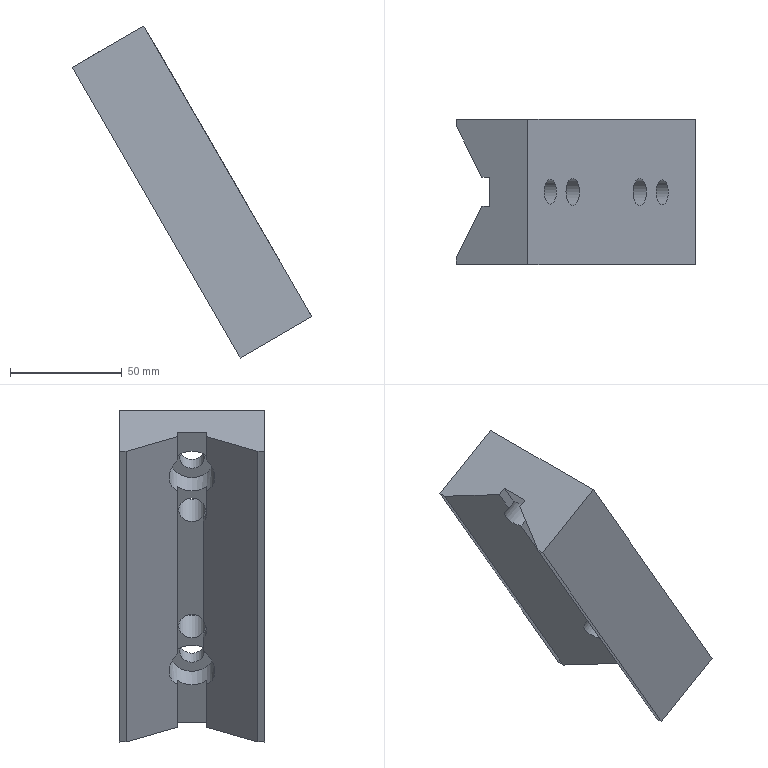Part | NX | features solid 2 | 1 solid | 30 faces | box 107.043 x 65 x 148.404 mm | volume 267589 mm3 | plane 22 | cylinder 8 | commonest cylinder face diameters 11 x2 12 x2 13 x2 20.5 x2
STEP:
#1=CARTESIAN_POINT('',(-1049.455,-56.5,78.567));
#2=VERTEX_POINT('',#1);
#3=CARTESIAN_POINT('',(-1043.418,-56.5,68.11));
#4=VERTEX_POINT('',#3);
#5=CARTESIAN_POINT('',(-1049.455,-56.5,78.567));
#6=DIRECTION('',(0.5,0.,-0.866));
#7=VECTOR('',#6,1000.);
#8=LINE('',#5,#7);
#9=EDGE_CURVE('',#2,#4,#8,.T.);
#10=ORIENTED_EDGE('',*,*,#9,.F.);
#11=CARTESIAN_POINT('',(-1049.455,-43.5,78.567));
#12=VERTEX_POINT('',#11);
#13=CARTESIAN_POINT('',(-1049.455,-82.5,78.567));
#14=DIRECTION('',(0.,-1.,0.));
#15=VECTOR('',#14,1000.);
#16=LINE('',#13,#15);
#17=EDGE_CURVE('',#12,#2,#16,.T.);
#18=ORIENTED_EDGE('',*,*,#17,.F.);
#19=CARTESIAN_POINT('',(-1043.418,-43.5,68.11));
#20=VERTEX_POINT('',#19);
#21=CARTESIAN_POINT('',(-1049.455,-43.5,78.567));
#22=DIRECTION('',(0.5,0.,-0.866));
#23=VECTOR('',#22,1000.);
#24=LINE('',#21,#23);
#25=EDGE_CURVE('',#12,#20,#24,.T.);
#26=ORIENTED_EDGE('',*,*,#25,.T.);
#27=CARTESIAN_POINT('',(-1039.455,-50.,61.247));
#28=DIRECTION('',(-0.866,0.,-0.5));
#29=DIRECTION('',(0.5,0.,-0.866));
#30=AXIS2_PLACEMENT_3D('',#27,#28,#29);
#31=CIRCLE('',#30,10.25);
#32=EDGE_CURVE('',#4,#20,#31,.T.);
#33=ORIENTED_EDGE('',*,*,#32,.F.);
#34=EDGE_LOOP('',(#10,#18,#26,#33));
#35=FACE_BOUND('',#34,.T.);
#36=CARTESIAN_POINT('',(-1049.455,-55.,78.567));
#37=DIRECTION('',(0.866,0.,0.5));
#38=DIRECTION('',(0.,-1.,0.));
#39=AXIS2_PLACEMENT_3D('',#36,#37,#38);
#40=PLANE('',#39);
#41=ADVANCED_FACE('',(#35),#40,.F.);
#42=CARTESIAN_POINT('',(-1046.668,-43.5,66.234));
#43=VERTEX_POINT('',#42);
#44=CARTESIAN_POINT('',(-1052.078,-43.5,63.11));
#45=DIRECTION('',(0.866,0.,0.5));
#46=VECTOR('',#45,1000.);
#47=LINE('',#44,#46);
#48=EDGE_CURVE('',#43,#20,#47,.T.);
#49=ORIENTED_EDGE('',*,*,#48,.T.);
#50=ORIENTED_EDGE('',*,*,#25,.F.);
#51=CARTESIAN_POINT('',(-1052.705,-43.5,76.691));
#52=VERTEX_POINT('',#51);
#53=CARTESIAN_POINT('',(-1050.223,-43.5,78.124));
#54=DIRECTION('',(0.866,0.,0.5));
#55=VECTOR('',#54,1000.);
#56=LINE('',#53,#55);
#57=EDGE_CURVE('',#52,#12,#56,.T.);
#58=ORIENTED_EDGE('',*,*,#57,.F.);
#59=CARTESIAN_POINT('',(-1052.705,-43.5,76.691));
#60=DIRECTION('',(0.5,0.,-0.866));
#61=VECTOR('',#60,1000.);
#62=LINE('',#59,#61);
#63=EDGE_CURVE('',#52,#43,#62,.T.);
#64=ORIENTED_EDGE('',*,*,#63,.T.);
#65=EDGE_LOOP('',(#49,#50,#58,#64));
#66=FACE_BOUND('',#65,.T.);
#67=CARTESIAN_POINT('',(-1050.223,-43.5,78.124));
#68=DIRECTION('',(0.,-1.,0.));
#69=DIRECTION('',(-0.866,0.,-0.5));
#70=AXIS2_PLACEMENT_3D('',#67,#68,#69);
#71=PLANE('',#70);
#72=ADVANCED_FACE('',(#66),#71,.T.);
#73=CARTESIAN_POINT('',(-1052.705,-56.5,76.691));
#74=VERTEX_POINT('',#73);
#75=CARTESIAN_POINT('',(-1046.668,-56.5,66.234));
#76=VERTEX_POINT('',#75);
#77=CARTESIAN_POINT('',(-1052.705,-56.5,76.691));
#78=DIRECTION('',(0.5,0.,-0.866));
#79=VECTOR('',#78,1000.);
#80=LINE('',#77,#79);
#81=EDGE_CURVE('',#74,#76,#80,.T.);
#82=ORIENTED_EDGE('',*,*,#81,.F.);
#83=CARTESIAN_POINT('',(-1050.223,-56.5,78.124));
#84=DIRECTION('',(0.866,0.,0.5));
#85=VECTOR('',#84,1000.);
#86=LINE('',#83,#85);
#87=EDGE_CURVE('',#74,#2,#86,.T.);
#88=ORIENTED_EDGE('',*,*,#87,.T.);
#89=ORIENTED_EDGE('',*,*,#9,.T.);
#90=CARTESIAN_POINT('',(-1052.078,-56.5,63.11));
#91=DIRECTION('',(0.866,0.,0.5));
#92=VECTOR('',#91,1000.);
#93=LINE('',#90,#92);
#94=EDGE_CURVE('',#76,#4,#93,.T.);
#95=ORIENTED_EDGE('',*,*,#94,.F.);
#96=EDGE_LOOP('',(#82,#88,#89,#95));
#97=FACE_BOUND('',#96,.T.);
#98=CARTESIAN_POINT('',(-1050.223,-56.5,78.124));
#99=DIRECTION('',(0.,-1.,0.));
#100=DIRECTION('',(-0.866,0.,-0.5));
#101=AXIS2_PLACEMENT_3D('',#98,#99,#100);
#102=PLANE('',#101);
#103=ADVANCED_FACE('',(#97),#102,.F.);
#104=CARTESIAN_POINT('',(-1038.743,-43.5,52.507));
#105=VERTEX_POINT('',#104);
#106=CARTESIAN_POINT('',(-1039.455,-50.,61.247));
#107=DIRECTION('',(0.75,0.5,0.433));
#108=DIRECTION('',(0.433,-0.866,0.25));
#109=AXIS2_PLACEMENT_3D('',#106,#107,#108);
#110=ELLIPSE('',#109,11.836,10.25);
#111=EDGE_CURVE('',#105,#43,#110,.T.);
#112=ORIENTED_EDGE('',*,*,#111,.T.);
#113=ORIENTED_EDGE('',*,*,#63,.F.);
#114=CARTESIAN_POINT('',(-1064.178,-20.555,70.067));
#115=VERTEX_POINT('',#114);
#116=CARTESIAN_POINT('',(-1064.178,-20.555,70.067));
#117=DIRECTION('',(0.433,-0.866,0.25));
#118=VECTOR('',#117,1000.);
#119=LINE('',#116,#118);
#120=EDGE_CURVE('',#115,#52,#119,.T.);
#121=ORIENTED_EDGE('',*,*,#120,.F.);
#122=CARTESIAN_POINT('',(-989.178,-20.555,-59.836));
#123=VERTEX_POINT('',#122);
#124=CARTESIAN_POINT('',(-1064.178,-20.555,70.067));
#125=DIRECTION('',(0.5,0.,-0.866));
#126=VECTOR('',#125,1000.);
#127=LINE('',#124,#126);
#128=EDGE_CURVE('',#115,#123,#127,.T.);
#129=ORIENTED_EDGE('',*,*,#128,.T.);
#130=CARTESIAN_POINT('',(-977.705,-43.5,-53.213));
#131=VERTEX_POINT('',#130);
#132=CARTESIAN_POINT('',(-987.509,-23.893,-58.873));
#133=DIRECTION('',(-0.433,0.866,-0.25));
#134=VECTOR('',#133,1000.);
#135=LINE('',#132,#134);
#136=EDGE_CURVE('',#123,#131,#135,.F.);
#137=ORIENTED_EDGE('',*,*,#136,.T.);
#138=CARTESIAN_POINT('',(-988.743,-43.5,-34.096));
#139=VERTEX_POINT('',#138);
#140=CARTESIAN_POINT('',(-1052.705,-43.5,76.691));
#141=DIRECTION('',(0.5,0.,-0.866));
#142=VECTOR('',#141,1000.);
#143=LINE('',#140,#142);
#144=EDGE_CURVE('',#139,#131,#143,.T.);
#145=ORIENTED_EDGE('',*,*,#144,.F.);
#146=CARTESIAN_POINT('',(-996.668,-43.5,-20.368));
#147=VERTEX_POINT('',#146);
#148=CARTESIAN_POINT('',(-989.455,-50.,-25.356));
#149=DIRECTION('',(0.75,0.5,0.433));
#150=DIRECTION('',(0.433,-0.866,0.25));
#151=AXIS2_PLACEMENT_3D('',#148,#149,#150);
#152=ELLIPSE('',#151,11.836,10.25);
#153=EDGE_CURVE('',#147,#139,#152,.F.);
#154=ORIENTED_EDGE('',*,*,#153,.F.);
#155=CARTESIAN_POINT('',(-1052.705,-43.5,76.691));
#156=DIRECTION('',(0.5,0.,-0.866));
#157=VECTOR('',#156,1000.);
#158=LINE('',#155,#157);
#159=EDGE_CURVE('',#105,#147,#158,.T.);
#160=ORIENTED_EDGE('',*,*,#159,.F.);
#161=EDGE_LOOP('',(#112,#113,#121,#129,#137,#145,#154,#160));
#162=FACE_BOUND('',#161,.T.);
#163=CARTESIAN_POINT('',(-1064.178,-20.555,70.067));
#164=DIRECTION('',(-0.75,-0.5,-0.433));
#165=DIRECTION('',(-0.433,0.866,-0.25));
#166=AXIS2_PLACEMENT_3D('',#163,#164,#165);
#167=PLANE('',#166);
#168=ADVANCED_FACE('',(#162),#167,.T.);
#169=ORIENTED_EDGE('',*,*,#144,.T.);
#170=CARTESIAN_POINT('',(-974.455,-43.5,-51.336));
#171=VERTEX_POINT('',#170);
#172=CARTESIAN_POINT('',(-976.187,-43.5,-52.336));
#173=DIRECTION('',(-0.866,0.,-0.5));
#174=VECTOR('',#173,1000.);
#175=LINE('',#172,#174);
#176=EDGE_CURVE('',#131,#171,#175,.F.);
#177=ORIENTED_EDGE('',*,*,#176,.T.);
#178=CARTESIAN_POINT('',(-985.493,-43.5,-32.219));
#179=VERTEX_POINT('',#178);
#180=CARTESIAN_POINT('',(-1049.455,-43.5,78.567));
#181=DIRECTION('',(0.5,0.,-0.866));
#182=VECTOR('',#181,1000.);
#183=LINE('',#180,#182);
#184=EDGE_CURVE('',#179,#171,#183,.T.);
#185=ORIENTED_EDGE('',*,*,#184,.F.);
#186=CARTESIAN_POINT('',(-988.743,-43.5,-34.096));
#187=DIRECTION('',(0.866,0.,0.5));
#188=VECTOR('',#187,1000.);
#189=LINE('',#186,#188);
#190=EDGE_CURVE('',#139,#179,#189,.T.);
#191=ORIENTED_EDGE('',*,*,#190,.F.);
#192=EDGE_LOOP('',(#169,#177,#185,#191));
#193=FACE_BOUND('',#192,.T.);
#194=CARTESIAN_POINT('',(-1050.223,-43.5,78.124));
#195=DIRECTION('',(0.,-1.,0.));
#196=DIRECTION('',(-0.866,0.,-0.5));
#197=AXIS2_PLACEMENT_3D('',#194,#195,#196);
#198=PLANE('',#197);
#199=ADVANCED_FACE('',(#193),#198,.T.);
#200=CARTESIAN_POINT('',(-993.929,-55.,-17.607));
#201=VERTEX_POINT('',#200);
#202=CARTESIAN_POINT('',(-996.429,-55.,-19.05));
#203=VERTEX_POINT('',#202);
#204=CARTESIAN_POINT('',(-1002.589,-55.,-22.607));
#205=DIRECTION('',(0.866,0.,0.5));
#206=VECTOR('',#205,1000.);
#207=LINE('',#204,#206);
#208=EDGE_CURVE('',#201,#203,#207,.F.);
#209=ORIENTED_EDGE('',*,*,#208,.T.);
#210=CARTESIAN_POINT('',(-999.879,-55.,-13.075));
#211=VERTEX_POINT('',#210);
#212=CARTESIAN_POINT('',(-1051.955,-55.,77.124));
#213=DIRECTION('',(0.5,0.,-0.866));
#214=VECTOR('',#213,1000.);
#215=LINE('',#212,#214);
#216=EDGE_CURVE('',#211,#203,#215,.T.);
#217=ORIENTED_EDGE('',*,*,#216,.F.);
#218=CARTESIAN_POINT('',(-997.379,-55.,-11.632));
#219=VERTEX_POINT('',#218);
#220=CARTESIAN_POINT('',(-993.049,-55.,-9.132));
#221=DIRECTION('',(-0.866,0.,-0.5));
#222=VECTOR('',#221,1000.);
#223=LINE('',#220,#222);
#224=EDGE_CURVE('',#211,#219,#223,.F.);
#225=ORIENTED_EDGE('',*,*,#224,.T.);
#226=CARTESIAN_POINT('',(-1049.455,-55.,78.567));
#227=DIRECTION('',(0.5,0.,-0.866));
#228=VECTOR('',#227,1000.);
#229=LINE('',#226,#228);
#230=EDGE_CURVE('',#219,#201,#229,.T.);
#231=ORIENTED_EDGE('',*,*,#230,.T.);
#232=EDGE_LOOP('',(#209,#217,#225,#231));
#233=FACE_BOUND('',#232,.T.);
#234=CARTESIAN_POINT('',(-1050.223,-55.,78.124));
#235=DIRECTION('',(0.,-1.,0.));
#236=DIRECTION('',(-0.866,0.,-0.5));
#237=AXIS2_PLACEMENT_3D('',#234,#235,#236);
#238=PLANE('',#237);
#239=ADVANCED_FACE('',(#233),#238,.F.);
#240=CARTESIAN_POINT('',(-988.743,-56.5,-34.096));
#241=VERTEX_POINT('',#240);
#242=CARTESIAN_POINT('',(-985.493,-56.5,-32.219));
#243=VERTEX_POINT('',#242);
#244=CARTESIAN_POINT('',(-994.153,-56.5,-37.219));
#245=DIRECTION('',(0.866,0.,0.5));
#246=VECTOR('',#245,1000.);
#247=LINE('',#244,#246);
#248=EDGE_CURVE('',#241,#243,#247,.T.);
#249=ORIENTED_EDGE('',*,*,#248,.T.);
#250=CARTESIAN_POINT('',(-974.455,-56.5,-51.336));
#251=VERTEX_POINT('',#250);
#252=CARTESIAN_POINT('',(-1049.455,-56.5,78.567));
#253=DIRECTION('',(0.5,0.,-0.866));
#254=VECTOR('',#253,1000.);
#255=LINE('',#252,#254);
#256=EDGE_CURVE('',#243,#251,#255,.T.);
#257=ORIENTED_EDGE('',*,*,#256,.T.);
#258=CARTESIAN_POINT('',(-977.705,-56.5,-53.213));
#259=VERTEX_POINT('',#258);
#260=CARTESIAN_POINT('',(-976.187,-56.5,-52.336));
#261=DIRECTION('',(-0.866,0.,-0.5));
#262=VECTOR('',#261,1000.);
#263=LINE('',#260,#262);
#264=EDGE_CURVE('',#259,#251,#263,.F.);
#265=ORIENTED_EDGE('',*,*,#264,.F.);
#266=CARTESIAN_POINT('',(-1052.705,-56.5,76.691));
#267=DIRECTION('',(0.5,0.,-0.866));
#268=VECTOR('',#267,1000.);
#269=LINE('',#266,#268);
#270=EDGE_CURVE('',#241,#259,#269,.T.);
#271=ORIENTED_EDGE('',*,*,#270,.F.);
#272=EDGE_LOOP('',(#249,#257,#265,#271));
#273=FACE_BOUND('',#272,.T.);
#274=CARTESIAN_POINT('',(-1050.223,-56.5,78.124));
#275=DIRECTION('',(0.,-1.,0.));
#276=DIRECTION('',(-0.866,0.,-0.5));
#277=AXIS2_PLACEMENT_3D('',#274,#275,#276);
#278=PLANE('',#277);
#279=ADVANCED_FACE('',(#273),#278,.F.);
#280=CARTESIAN_POINT('',(-1038.743,-56.5,52.507));
#281=VERTEX_POINT('',#280);
#282=CARTESIAN_POINT('',(-1032.705,-56.5,42.05));
#283=VERTEX_POINT('',#282);
#284=CARTESIAN_POINT('',(-1052.705,-56.5,76.691));
#285=DIRECTION('',(0.5,0.,-0.866));
#286=VECTOR('',#285,1000.);
#287=LINE('',#284,#286);
#288=EDGE_CURVE('',#281,#283,#287,.T.);
#289=ORIENTED_EDGE('',*,*,#288,.T.);
#290=CARTESIAN_POINT('',(-1029.879,-55.,38.886));
#291=VERTEX_POINT('',#290);
#292=CARTESIAN_POINT('',(-1029.455,-50.,43.926));
#293=DIRECTION('',(-0.75,0.5,-0.433));
#294=DIRECTION('',(-0.433,-0.866,-0.25));
#295=AXIS2_PLACEMENT_3D('',#292,#293,#294);
#296=ELLIPSE('',#295,7.506,6.5);
#297=EDGE_CURVE('',#283,#291,#296,.F.);
#298=ORIENTED_EDGE('',*,*,#297,.T.);
#299=CARTESIAN_POINT('',(-1004.032,-55.,-5.882));
#300=VERTEX_POINT('',#299);
#301=CARTESIAN_POINT('',(-1051.955,-55.,77.124));
#302=DIRECTION('',(0.5,0.,-0.866));
#303=VECTOR('',#302,1000.);
#304=LINE('',#301,#303);
#305=EDGE_CURVE('',#291,#300,#304,.T.);
#306=ORIENTED_EDGE('',*,*,#305,.T.);
#307=CARTESIAN_POINT('',(-999.455,-50.,-8.035));
#308=DIRECTION('',(-0.75,0.5,-0.433));
#309=DIRECTION('',(-0.433,-0.866,-0.25));
#310=AXIS2_PLACEMENT_3D('',#307,#308,#309);
#311=ELLIPSE('',#310,7.506,6.5);
#312=EDGE_CURVE('',#300,#211,#311,.F.);
#313=ORIENTED_EDGE('',*,*,#312,.T.);
#314=ORIENTED_EDGE('',*,*,#216,.T.);
#315=CARTESIAN_POINT('',(-989.455,-50.,-25.356));
#316=DIRECTION('',(-0.75,0.5,-0.433));
#317=DIRECTION('',(0.433,0.866,0.25));
#318=AXIS2_PLACEMENT_3D('',#315,#316,#317);
#319=ELLIPSE('',#318,11.836,10.25);
#320=EDGE_CURVE('',#203,#241,#319,.F.);
#321=ORIENTED_EDGE('',*,*,#320,.T.);
#322=ORIENTED_EDGE('',*,*,#270,.T.);
#323=CARTESIAN_POINT('',(-989.178,-79.445,-59.836));
#324=VERTEX_POINT('',#323);
#325=CARTESIAN_POINT('',(-962.701,-26.491,-44.55));
#326=DIRECTION('',(-0.433,-0.866,-0.25));
#327=VECTOR('',#326,1000.);
#328=LINE('',#325,#327);
#329=EDGE_CURVE('',#324,#259,#328,.F.);
#330=ORIENTED_EDGE('',*,*,#329,.F.);
#331=CARTESIAN_POINT('',(-1064.178,-79.445,70.067));
#332=VERTEX_POINT('',#331);
#333=CARTESIAN_POINT('',(-1064.178,-79.445,70.067));
#334=DIRECTION('',(-0.5,0.,0.866));
#335=VECTOR('',#334,1000.);
#336=LINE('',#333,#335);
#337=EDGE_CURVE('',#332,#324,#336,.F.);
#338=ORIENTED_EDGE('',*,*,#337,.F.);
#339=CARTESIAN_POINT('',(-1064.178,-79.445,70.067));
#340=DIRECTION('',(0.433,0.866,0.25));
#341=VECTOR('',#340,1000.);
#342=LINE('',#339,#341);
#343=EDGE_CURVE('',#332,#74,#342,.T.);
#344=ORIENTED_EDGE('',*,*,#343,.T.);
#345=ORIENTED_EDGE('',*,*,#81,.T.);
#346=CARTESIAN_POINT('',(-1039.455,-50.,61.247));
#347=DIRECTION('',(-0.75,0.5,-0.433));
#348=DIRECTION('',(0.433,0.866,0.25));
#349=AXIS2_PLACEMENT_3D('',#346,#347,#348);
#350=ELLIPSE('',#349,11.836,10.25);
#351=EDGE_CURVE('',#281,#76,#350,.T.);
#352=ORIENTED_EDGE('',*,*,#351,.F.);
#353=EDGE_LOOP('',(#289,#298,#306,#313,#314,#321,#322,#330,#338,#344,#345,#352));
#354=FACE_BOUND('',#353,.T.);
#355=CARTESIAN_POINT('',(-1064.178,-79.445,70.067));
#356=DIRECTION('',(0.75,-0.5,0.433));
#357=DIRECTION('',(-0.433,-0.866,-0.25));
#358=AXIS2_PLACEMENT_3D('',#355,#356,#357);
#359=PLANE('',#358);
#360=ADVANCED_FACE('',(#354),#359,.F.);
#361=CARTESIAN_POINT('',(-989.455,-50.,-25.356));
#362=DIRECTION('',(-0.866,0.,-0.5));
#363=DIRECTION('',(0.5,0.,-0.866));
#364=AXIS2_PLACEMENT_3D('',#361,#362,#363);
#365=CIRCLE('',#364,10.25);
#366=EDGE_CURVE('',#243,#179,#365,.F.);
#367=ORIENTED_EDGE('',*,*,#366,.T.);
#368=ORIENTED_EDGE('',*,*,#184,.T.);
#369=CARTESIAN_POINT('',(-974.455,-17.5,-51.336));
#370=DIRECTION('',(0.,-1.,0.));
#371=VECTOR('',#370,1000.);
#372=LINE('',#369,#371);
#373=EDGE_CURVE('',#251,#171,#372,.F.);
#374=ORIENTED_EDGE('',*,*,#373,.F.);
#375=ORIENTED_EDGE('',*,*,#256,.F.);
#376=EDGE_LOOP('',(#367,#368,#374,#375));
#377=FACE_BOUND('',#376,.T.);
#378=CARTESIAN_POINT('',(-1049.455,-55.,78.567));
#379=DIRECTION('',(0.866,0.,0.5));
#380=DIRECTION('',(0.,-1.,0.));
#381=AXIS2_PLACEMENT_3D('',#378,#379,#380);
#382=PLANE('',#381);
#383=ADVANCED_FACE('',(#377),#382,.F.);
#384=CARTESIAN_POINT('',(-1026.455,-50.,38.73));
#385=VERTEX_POINT('',#384);
#386=CARTESIAN_POINT('',(-1029.455,-50.,43.926));
#387=DIRECTION('',(-0.866,0.,-0.5));
#388=DIRECTION('',(0.5,0.,-0.866));
#389=AXIS2_PLACEMENT_3D('',#386,#387,#388);
#390=CIRCLE('',#389,6.);
#391=EDGE_CURVE('',#385,#385,#390,.T.);
#392=ORIENTED_EDGE('',*,*,#391,.F.);
#393=EDGE_LOOP('',(#392));
#394=FACE_BOUND('',#393,.T.);
#395=CARTESIAN_POINT('',(-996.455,-50.,-13.231));
#396=VERTEX_POINT('',#395);
#397=CARTESIAN_POINT('',(-999.455,-50.,-8.035));
#398=DIRECTION('',(-0.866,0.,-0.5));
#399=DIRECTION('',(0.5,0.,-0.866));
#400=AXIS2_PLACEMENT_3D('',#397,#398,#399);
#401=CIRCLE('',#400,6.);
#402=EDGE_CURVE('',#396,#396,#401,.T.);
#403=ORIENTED_EDGE('',*,*,#402,.F.);
#404=EDGE_LOOP('',(#403));
#405=FACE_BOUND('',#404,.T.);
#406=CARTESIAN_POINT('',(-1035.493,-43.5,54.383));
#407=VERTEX_POINT('',#406);
#408=CARTESIAN_POINT('',(-993.418,-43.5,-18.492));
#409=VERTEX_POINT('',#408);
#410=CARTESIAN_POINT('',(-1049.455,-43.5,78.567));
#411=DIRECTION('',(0.5,0.,-0.866));
#412=VECTOR('',#411,1000.);
#413=LINE('',#410,#412);
#414=EDGE_CURVE('',#407,#409,#413,.T.);
#415=ORIENTED_EDGE('',*,*,#414,.T.);
#416=CARTESIAN_POINT('',(-989.455,-50.,-25.356));
#417=DIRECTION('',(-0.866,0.,-0.5));
#418=DIRECTION('',(0.5,0.,-0.866));
#419=AXIS2_PLACEMENT_3D('',#416,#417,#418);
#420=CIRCLE('',#419,10.25);
#421=EDGE_CURVE('',#409,#201,#420,.F.);
#422=ORIENTED_EDGE('',*,*,#421,.T.);
#423=ORIENTED_EDGE('',*,*,#230,.F.);
#424=CARTESIAN_POINT('',(-1001.532,-55.,-4.438));
#425=VERTEX_POINT('',#424);
#426=CARTESIAN_POINT('',(-999.455,-50.,-8.035));
#427=DIRECTION('',(-0.866,0.,-0.5));
#428=DIRECTION('',(0.5,0.,-0.866));
#429=AXIS2_PLACEMENT_3D('',#426,#427,#428);
#430=CIRCLE('',#429,6.5);
#431=EDGE_CURVE('',#219,#425,#430,.T.);
#432=ORIENTED_EDGE('',*,*,#431,.T.);
#433=CARTESIAN_POINT('',(-1027.379,-55.,40.329));
#434=VERTEX_POINT('',#433);
#435=CARTESIAN_POINT('',(-1049.455,-55.,78.567));
#436=DIRECTION('',(0.5,0.,-0.866));
#437=VECTOR('',#436,1000.);
#438=LINE('',#435,#437);
#439=EDGE_CURVE('',#434,#425,#438,.T.);
#440=ORIENTED_EDGE('',*,*,#439,.F.);
#441=CARTESIAN_POINT('',(-1029.455,-56.5,43.926));
#442=VERTEX_POINT('',#441);
#443=CARTESIAN_POINT('',(-1029.455,-50.,43.926));
#444=DIRECTION('',(-0.866,0.,-0.5));
#445=DIRECTION('',(0.5,0.,-0.866));
#446=AXIS2_PLACEMENT_3D('',#443,#444,#445);
#447=CIRCLE('',#446,6.5);
#448=EDGE_CURVE('',#434,#442,#447,.T.);
#449=ORIENTED_EDGE('',*,*,#448,.T.);
#450=CARTESIAN_POINT('',(-1035.493,-56.5,54.383));
#451=VERTEX_POINT('',#450);
#452=CARTESIAN_POINT('',(-1049.455,-56.5,78.567));
#453=DIRECTION('',(0.5,0.,-0.866));
#454=VECTOR('',#453,1000.);
#455=LINE('',#452,#454);
#456=EDGE_CURVE('',#451,#442,#455,.T.);
#457=ORIENTED_EDGE('',*,*,#456,.F.);
#458=CARTESIAN_POINT('',(-1039.455,-50.,61.247));
#459=DIRECTION('',(-0.866,0.,-0.5));
#460=DIRECTION('',(0.5,0.,-0.866));
#461=AXIS2_PLACEMENT_3D('',#458,#459,#460);
#462=CIRCLE('',#461,10.25);
#463=EDGE_CURVE('',#407,#451,#462,.T.);
#464=ORIENTED_EDGE('',*,*,#463,.F.);
#465=EDGE_LOOP('',(#415,#422,#423,#432,#440,#449,#457,#464));
#466=FACE_BOUND('',#465,.T.);
#467=CARTESIAN_POINT('',(-1049.455,-55.,78.567));
#468=DIRECTION('',(0.866,0.,0.5));
#469=DIRECTION('',(0.,-1.,0.));
#470=AXIS2_PLACEMENT_3D('',#467,#468,#469);
#471=PLANE('',#470);
#472=ADVANCED_FACE('',(#394,#405,#466),#471,.F.);
#473=CARTESIAN_POINT('',(-1022.135,-44.5,71.247));
#474=VERTEX_POINT('',#473);
#475=CARTESIAN_POINT('',(-1022.135,-50.,71.247));
#476=DIRECTION('',(-0.866,0.,-0.5));
#477=DIRECTION('',(0.,1.,0.));
#478=AXIS2_PLACEMENT_3D('',#475,#476,#477);
#479=CIRCLE('',#478,5.5);
#480=EDGE_CURVE('',#474,#474,#479,.T.);
#481=ORIENTED_EDGE('',*,*,#480,.T.);
#482=EDGE_LOOP('',(#481));
#483=FACE_BOUND('',#482,.T.);
#484=CARTESIAN_POINT('',(-957.135,-82.5,-41.336));
#485=VERTEX_POINT('',#484);
#486=CARTESIAN_POINT('',(-957.135,-17.5,-41.336));
#487=VERTEX_POINT('',#486);
#488=CARTESIAN_POINT('',(-957.135,-17.5,-41.336));
#489=DIRECTION('',(0.,-1.,0.));
#490=VECTOR('',#489,1000.);
#491=LINE('',#488,#490);
#492=EDGE_CURVE('',#485,#487,#491,.F.);
#493=ORIENTED_EDGE('',*,*,#492,.T.);
#494=CARTESIAN_POINT('',(-1032.135,-17.5,88.567));
#495=VERTEX_POINT('',#494);
#496=CARTESIAN_POINT('',(-1032.135,-17.5,88.567));
#497=DIRECTION('',(0.5,0.,-0.866));
#498=VECTOR('',#497,1000.);
#499=LINE('',#496,#498);
#500=EDGE_CURVE('',#495,#487,#499,.T.);
#501=ORIENTED_EDGE('',*,*,#500,.F.);
#502=CARTESIAN_POINT('',(-1032.135,-82.5,88.567));
#503=VERTEX_POINT('',#502);
#504=CARTESIAN_POINT('',(-1032.135,-50.,88.567));
#505=DIRECTION('',(0.,-1.,0.));
#506=VECTOR('',#505,1000.);
#507=LINE('',#504,#506);
#508=EDGE_CURVE('',#495,#503,#507,.T.);
#509=ORIENTED_EDGE('',*,*,#508,.T.);
#510=CARTESIAN_POINT('',(-1032.135,-82.5,88.567));
#511=DIRECTION('',(0.5,0.,-0.866));
#512=VECTOR('',#511,1000.);
#513=LINE('',#510,#512);
#514=EDGE_CURVE('',#503,#485,#513,.T.);
#515=ORIENTED_EDGE('',*,*,#514,.T.);
#516=EDGE_LOOP('',(#493,#501,#509,#515));
#517=FACE_BOUND('',#516,.T.);
#518=CARTESIAN_POINT('',(-1009.135,-50.,48.73));
#519=VERTEX_POINT('',#518);
#520=CARTESIAN_POINT('',(-1012.135,-50.,53.926));
#521=DIRECTION('',(-0.866,0.,-0.5));
#522=DIRECTION('',(0.5,0.,-0.866));
#523=AXIS2_PLACEMENT_3D('',#520,#521,#522);
#524=CIRCLE('',#523,6.);
#525=EDGE_CURVE('',#519,#519,#524,.F.);
#526=ORIENTED_EDGE('',*,*,#525,.F.);
#527=EDGE_LOOP('',(#526));
#528=FACE_BOUND('',#527,.T.);
#529=CARTESIAN_POINT('',(-979.135,-50.,-3.231));
#530=VERTEX_POINT('',#529);
#531=CARTESIAN_POINT('',(-982.135,-50.,1.965));
#532=DIRECTION('',(-0.866,0.,-0.5));
#533=DIRECTION('',(0.5,0.,-0.866));
#534=AXIS2_PLACEMENT_3D('',#531,#532,#533);
#535=CIRCLE('',#534,6.);
#536=EDGE_CURVE('',#530,#530,#535,.F.);
#537=ORIENTED_EDGE('',*,*,#536,.F.);
#538=EDGE_LOOP('',(#537));
#539=FACE_BOUND('',#538,.T.);
#540=CARTESIAN_POINT('',(-972.135,-44.5,-15.356));
#541=VERTEX_POINT('',#540);
#542=CARTESIAN_POINT('',(-972.135,-50.,-15.356));
#543=DIRECTION('',(0.866,0.,0.5));
#544=DIRECTION('',(0.,1.,0.));
#545=AXIS2_PLACEMENT_3D('',#542,#543,#544);
#546=CIRCLE('',#545,5.5);
#547=EDGE_CURVE('',#541,#541,#546,.T.);
#548=ORIENTED_EDGE('',*,*,#547,.F.);
#549=EDGE_LOOP('',(#548));
#550=FACE_BOUND('',#549,.T.);
#551=CARTESIAN_POINT('',(-1032.135,-50.,88.567));
#552=DIRECTION('',(0.866,0.,0.5));
#553=DIRECTION('',(0.,-1.,0.));
#554=AXIS2_PLACEMENT_3D('',#551,#552,#553);
#555=PLANE('',#554);
#556=ADVANCED_FACE('',(#483,#517,#528,#539,#550),#555,.T.);
#557=CARTESIAN_POINT('',(-997.202,-55.,-1.938));
#558=DIRECTION('',(-0.866,0.,-0.5));
#559=VECTOR('',#558,1000.);
#560=LINE('',#557,#559);
#561=EDGE_CURVE('',#425,#300,#560,.T.);
#562=ORIENTED_EDGE('',*,*,#561,.T.);
#563=ORIENTED_EDGE('',*,*,#305,.F.);
#564=CARTESIAN_POINT('',(-1023.049,-55.,42.829));
#565=DIRECTION('',(-0.866,0.,-0.5));
#566=VECTOR('',#565,1000.);
#567=LINE('',#564,#566);
#568=EDGE_CURVE('',#291,#434,#567,.F.);
#569=ORIENTED_EDGE('',*,*,#568,.T.);
#570=ORIENTED_EDGE('',*,*,#439,.T.);
#571=EDGE_LOOP('',(#562,#563,#569,#570));
#572=FACE_BOUND('',#571,.T.);
#573=CARTESIAN_POINT('',(-1050.223,-55.,78.124));
#574=DIRECTION('',(0.,-1.,0.));
#575=DIRECTION('',(-0.866,0.,-0.5));
#576=AXIS2_PLACEMENT_3D('',#573,#574,#575);
#577=PLANE('',#576);
#578=ADVANCED_FACE('',(#572),#577,.F.);
#579=CARTESIAN_POINT('',(-1044.153,-43.5,49.383));
#580=DIRECTION('',(0.866,0.,0.5));
#581=VECTOR('',#580,1000.);
#582=LINE('',#579,#581);
#583=EDGE_CURVE('',#407,#105,#582,.F.);
#584=ORIENTED_EDGE('',*,*,#583,.T.);
#585=ORIENTED_EDGE('',*,*,#159,.T.);
#586=CARTESIAN_POINT('',(-989.088,-43.5,-15.992));
#587=DIRECTION('',(0.866,0.,0.5));
#588=VECTOR('',#587,1000.);
#589=LINE('',#586,#588);
#590=EDGE_CURVE('',#409,#147,#589,.F.);
#591=ORIENTED_EDGE('',*,*,#590,.F.);
#592=ORIENTED_EDGE('',*,*,#414,.F.);
#593=EDGE_LOOP('',(#584,#585,#591,#592));
#594=FACE_BOUND('',#593,.T.);
#595=CARTESIAN_POINT('',(-1050.223,-43.5,78.124));
#596=DIRECTION('',(0.,-1.,0.));
#597=DIRECTION('',(-0.866,0.,-0.5));
#598=AXIS2_PLACEMENT_3D('',#595,#596,#597);
#599=PLANE('',#598);
#600=ADVANCED_FACE('',(#594),#599,.T.);
#601=ORIENTED_EDGE('',*,*,#456,.T.);
#602=CARTESIAN_POINT('',(-1028.54,-56.5,44.455));
#603=DIRECTION('',(-0.866,0.,-0.5));
#604=VECTOR('',#603,1000.);
#605=LINE('',#602,#604);
#606=EDGE_CURVE('',#442,#283,#605,.T.);
#607=ORIENTED_EDGE('',*,*,#606,.T.);
#608=ORIENTED_EDGE('',*,*,#288,.F.);
#609=CARTESIAN_POINT('',(-1044.153,-56.5,49.383));
#610=DIRECTION('',(0.866,0.,0.5));
#611=VECTOR('',#610,1000.);
#612=LINE('',#609,#611);
#613=EDGE_CURVE('',#451,#281,#612,.F.);
#614=ORIENTED_EDGE('',*,*,#613,.F.);
#615=EDGE_LOOP('',(#601,#607,#608,#614));
#616=FACE_BOUND('',#615,.T.);
#617=CARTESIAN_POINT('',(-1050.223,-56.5,78.124));
#618=DIRECTION('',(0.,-1.,0.));
#619=DIRECTION('',(-0.866,0.,-0.5));
#620=AXIS2_PLACEMENT_3D('',#617,#618,#619);
#621=PLANE('',#620);
#622=ADVANCED_FACE('',(#616),#621,.F.);
#623=CARTESIAN_POINT('',(-989.178,-17.5,-59.836));
#624=VERTEX_POINT('',#623);
#625=CARTESIAN_POINT('',(-989.178,-17.5,-59.836));
#626=DIRECTION('',(0.,1.,0.));
#627=VECTOR('',#626,1000.);
#628=LINE('',#625,#627);
#629=EDGE_CURVE('',#624,#123,#628,.F.);
#630=ORIENTED_EDGE('',*,*,#629,.T.);
#631=ORIENTED_EDGE('',*,*,#128,.F.);
#632=CARTESIAN_POINT('',(-1064.178,-17.5,70.067));
#633=VERTEX_POINT('',#632);
#634=CARTESIAN_POINT('',(-1064.178,-17.5,70.067));
#635=DIRECTION('',(0.,-1.,0.));
#636=VECTOR('',#635,1000.);
#637=LINE('',#634,#636);
#638=EDGE_CURVE('',#633,#115,#637,.T.);
#639=ORIENTED_EDGE('',*,*,#638,.F.);
#640=CARTESIAN_POINT('',(-1064.178,-17.5,70.067));
#641=DIRECTION('',(0.5,0.,-0.866));
#642=VECTOR('',#641,1000.);
#643=LINE('',#640,#642);
#644=EDGE_CURVE('',#633,#624,#643,.T.);
#645=ORIENTED_EDGE('',*,*,#644,.T.);
#646=EDGE_LOOP('',(#630,#631,#639,#645));
#647=FACE_BOUND('',#646,.T.);
#648=CARTESIAN_POINT('',(-1064.178,-17.5,70.067));
#649=DIRECTION('',(-0.866,0.,-0.5));
#650=DIRECTION('',(0.,1.,0.));
#651=AXIS2_PLACEMENT_3D('',#648,#649,#650);
#652=PLANE('',#651);
#653=ADVANCED_FACE('',(#647),#652,.T.);
#654=CARTESIAN_POINT('',(-989.178,-82.5,-59.836));
#655=VERTEX_POINT('',#654);
#656=CARTESIAN_POINT('',(-989.178,-17.5,-59.836));
#657=DIRECTION('',(0.,1.,0.));
#658=VECTOR('',#657,1000.);
#659=LINE('',#656,#658);
#660=EDGE_CURVE('',#655,#324,#659,.T.);
#661=ORIENTED_EDGE('',*,*,#660,.F.);
#662=CARTESIAN_POINT('',(-1064.178,-82.5,70.067));
#663=VERTEX_POINT('',#662);
#664=CARTESIAN_POINT('',(-1064.178,-82.5,70.067));
#665=DIRECTION('',(-0.5,0.,0.866));
#666=VECTOR('',#665,1000.);
#667=LINE('',#664,#666);
#668=EDGE_CURVE('',#663,#655,#667,.F.);
#669=ORIENTED_EDGE('',*,*,#668,.F.);
#670=CARTESIAN_POINT('',(-1064.178,-17.5,70.067));
#671=DIRECTION('',(0.,-1.,0.));
#672=VECTOR('',#671,1000.);
#673=LINE('',#670,#672);
#674=EDGE_CURVE('',#663,#332,#673,.F.);
#675=ORIENTED_EDGE('',*,*,#674,.T.);
#676=ORIENTED_EDGE('',*,*,#337,.T.);
#677=EDGE_LOOP('',(#661,#669,#675,#676));
#678=FACE_BOUND('',#677,.T.);
#679=CARTESIAN_POINT('',(-1064.178,-17.5,70.067));
#680=DIRECTION('',(-0.866,0.,-0.5));
#681=DIRECTION('',(0.,1.,0.));
#682=AXIS2_PLACEMENT_3D('',#679,#680,#681);
#683=PLANE('',#682);
#684=ADVANCED_FACE('',(#678),#683,.T.);
#685=CARTESIAN_POINT('',(-976.187,-82.5,-52.336));
#686=DIRECTION('',(0.866,0.,0.5));
#687=VECTOR('',#686,1000.);
#688=LINE('',#685,#687);
#689=EDGE_CURVE('',#485,#655,#688,.F.);
#690=ORIENTED_EDGE('',*,*,#689,.F.);
#691=ORIENTED_EDGE('',*,*,#514,.F.);
#692=CARTESIAN_POINT('',(-1032.135,-82.5,88.567));
#693=DIRECTION('',(-0.866,0.,-0.5));
#694=VECTOR('',#693,1000.);
#695=LINE('',#692,#694);
#696=EDGE_CURVE('',#503,#663,#695,.T.);
#697=ORIENTED_EDGE('',*,*,#696,.T.);
#698=ORIENTED_EDGE('',*,*,#668,.T.);
#699=EDGE_LOOP('',(#690,#691,#697,#698));
#700=FACE_BOUND('',#699,.T.);
#701=CARTESIAN_POINT('',(-1032.135,-82.5,88.567));
#702=DIRECTION('',(0.,1.,0.));
#703=DIRECTION('',(0.866,0.,0.5));
#704=AXIS2_PLACEMENT_3D('',#701,#702,#703);
#705=PLANE('',#704);
#706=ADVANCED_FACE('',(#700),#705,.F.);
#707=CARTESIAN_POINT('',(-976.187,-17.5,-52.336));
#708=DIRECTION('',(0.866,0.,0.5));
#709=VECTOR('',#708,1000.);
#710=LINE('',#707,#709);
#711=EDGE_CURVE('',#487,#624,#710,.F.);
#712=ORIENTED_EDGE('',*,*,#711,.T.);
#713=ORIENTED_EDGE('',*,*,#644,.F.);
#714=CARTESIAN_POINT('',(-1032.135,-17.5,88.567));
#715=DIRECTION('',(-0.866,0.,-0.5));
#716=VECTOR('',#715,1000.);
#717=LINE('',#714,#716);
#718=EDGE_CURVE('',#495,#633,#717,.T.);
#719=ORIENTED_EDGE('',*,*,#718,.F.);
#720=ORIENTED_EDGE('',*,*,#500,.T.);
#721=EDGE_LOOP('',(#712,#713,#719,#720));
#722=FACE_BOUND('',#721,.T.);
#723=CARTESIAN_POINT('',(-1032.135,-17.5,88.567));
#724=DIRECTION('',(0.,1.,0.));
#725=DIRECTION('',(0.866,0.,0.5));
#726=AXIS2_PLACEMENT_3D('',#723,#724,#725);
#727=PLANE('',#726);
#728=ADVANCED_FACE('',(#722),#727,.T.);
#729=ORIENTED_EDGE('',*,*,#638,.T.);
#730=ORIENTED_EDGE('',*,*,#120,.T.);
#731=ORIENTED_EDGE('',*,*,#57,.T.);
#732=ORIENTED_EDGE('',*,*,#17,.T.);
#733=ORIENTED_EDGE('',*,*,#87,.F.);
#734=ORIENTED_EDGE('',*,*,#343,.F.);
#735=ORIENTED_EDGE('',*,*,#674,.F.);
#736=ORIENTED_EDGE('',*,*,#696,.F.);
#737=ORIENTED_EDGE('',*,*,#508,.F.);
#738=ORIENTED_EDGE('',*,*,#718,.T.);
#739=EDGE_LOOP('',(#729,#730,#731,#732,#733,#734,#735,#736,#737,#738));
#740=FACE_BOUND('',#739,.T.);
#741=CARTESIAN_POINT('',(-1062.446,-82.5,71.067));
#742=DIRECTION('',(-0.5,0.,0.866));
#743=DIRECTION('',(-0.866,0.,-0.5));
#744=AXIS2_PLACEMENT_3D('',#741,#742,#743);
#745=PLANE('',#744);
#746=ADVANCED_FACE('',(#740),#745,.T.);
#747=ORIENTED_EDGE('',*,*,#629,.F.);
#748=ORIENTED_EDGE('',*,*,#711,.F.);
#749=ORIENTED_EDGE('',*,*,#492,.F.);
#750=ORIENTED_EDGE('',*,*,#689,.T.);
#751=ORIENTED_EDGE('',*,*,#660,.T.);
#752=ORIENTED_EDGE('',*,*,#329,.T.);
#753=ORIENTED_EDGE('',*,*,#264,.T.);
#754=ORIENTED_EDGE('',*,*,#373,.T.);
#755=ORIENTED_EDGE('',*,*,#176,.F.);
#756=ORIENTED_EDGE('',*,*,#136,.F.);
#757=EDGE_LOOP('',(#747,#748,#749,#750,#751,#752,#753,#754,#755,#756));
#758=FACE_BOUND('',#757,.T.);
#759=CARTESIAN_POINT('',(-976.187,-17.5,-52.336));
#760=DIRECTION('',(-0.5,0.,0.866));
#761=DIRECTION('',(0.,1.,0.));
#762=AXIS2_PLACEMENT_3D('',#759,#760,#761);
#763=PLANE('',#762);
#764=ADVANCED_FACE('',(#758),#763,.F.);
#765=ORIENTED_EDGE('',*,*,#525,.T.);
#766=EDGE_LOOP('',(#765));
#767=FACE_BOUND('',#766,.T.);
#768=ORIENTED_EDGE('',*,*,#391,.T.);
#769=EDGE_LOOP('',(#768));
#770=FACE_BOUND('',#769,.T.);
#771=CARTESIAN_POINT('',(-1012.135,-50.,53.926));
#772=DIRECTION('',(-0.866,0.,-0.5));
#773=DIRECTION('',(0.,1.,0.));
#774=AXIS2_PLACEMENT_3D('',#771,#772,#773);
#775=CYLINDRICAL_SURFACE('',#774,6.);
#776=ADVANCED_FACE('',(#767,#770),#775,.F.);
#777=ORIENTED_EDGE('',*,*,#536,.T.);
#778=EDGE_LOOP('',(#777));
#779=FACE_BOUND('',#778,.T.);
#780=ORIENTED_EDGE('',*,*,#402,.T.);
#781=EDGE_LOOP('',(#780));
#782=FACE_BOUND('',#781,.T.);
#783=CARTESIAN_POINT('',(-982.135,-50.,1.965));
#784=DIRECTION('',(-0.866,0.,-0.5));
#785=DIRECTION('',(0.,1.,0.));
#786=AXIS2_PLACEMENT_3D('',#783,#784,#785);
#787=CYLINDRICAL_SURFACE('',#786,6.);
#788=ADVANCED_FACE('',(#779,#782),#787,.F.);
#789=ORIENTED_EDGE('',*,*,#568,.F.);
#790=ORIENTED_EDGE('',*,*,#297,.F.);
#791=ORIENTED_EDGE('',*,*,#606,.F.);
#792=ORIENTED_EDGE('',*,*,#448,.F.);
#793=EDGE_LOOP('',(#789,#790,#791,#792));
#794=FACE_BOUND('',#793,.T.);
#795=CARTESIAN_POINT('',(-1025.125,-50.,46.426));
#796=DIRECTION('',(-0.866,0.,-0.5));
#797=DIRECTION('',(0.,1.,0.));
#798=AXIS2_PLACEMENT_3D('',#795,#796,#797);
#799=CYLINDRICAL_SURFACE('',#798,6.5);
#800=ADVANCED_FACE('',(#794),#799,.F.);
#801=ORIENTED_EDGE('',*,*,#224,.F.);
#802=ORIENTED_EDGE('',*,*,#312,.F.);
#803=ORIENTED_EDGE('',*,*,#561,.F.);
#804=ORIENTED_EDGE('',*,*,#431,.F.);
#805=EDGE_LOOP('',(#801,#802,#803,#804));
#806=FACE_BOUND('',#805,.T.);
#807=CARTESIAN_POINT('',(-995.125,-50.,-5.535));
#808=DIRECTION('',(-0.866,0.,-0.5));
#809=DIRECTION('',(0.,1.,0.));
#810=AXIS2_PLACEMENT_3D('',#807,#808,#809);
#811=CYLINDRICAL_SURFACE('',#810,6.5);
#812=ADVANCED_FACE('',(#806),#811,.F.);
#813=CARTESIAN_POINT('',(-979.063,-44.5,-19.356));
#814=VERTEX_POINT('',#813);
#815=CARTESIAN_POINT('',(-979.063,-50.,-19.356));
#816=DIRECTION('',(0.866,0.,0.5));
#817=DIRECTION('',(0.,1.,0.));
#818=AXIS2_PLACEMENT_3D('',#815,#816,#817);
#819=CIRCLE('',#818,5.5);
#820=EDGE_CURVE('',#814,#814,#819,.T.);
#821=ORIENTED_EDGE('',*,*,#820,.F.);
#822=EDGE_LOOP('',(#821));
#823=FACE_BOUND('',#822,.T.);
#824=ORIENTED_EDGE('',*,*,#547,.T.);
#825=EDGE_LOOP('',(#824));
#826=FACE_BOUND('',#825,.T.);
#827=CARTESIAN_POINT('',(-979.063,-50.,-19.356));
#828=DIRECTION('',(0.866,0.,0.5));
#829=DIRECTION('',(0.,-1.,0.));
#830=AXIS2_PLACEMENT_3D('',#827,#828,#829);
#831=CYLINDRICAL_SURFACE('',#830,5.5);
#832=ADVANCED_FACE('',(#823,#826),#831,.F.);
#833=CARTESIAN_POINT('',(-1029.063,-55.5,67.247));
#834=VERTEX_POINT('',#833);
#835=CARTESIAN_POINT('',(-1029.063,-50.,67.247));
#836=DIRECTION('',(-0.866,0.,-0.5));
#837=DIRECTION('',(0.,-1.,0.));
#838=AXIS2_PLACEMENT_3D('',#835,#836,#837);
#839=CIRCLE('',#838,5.5);
#840=EDGE_CURVE('',#834,#834,#839,.F.);
#841=ORIENTED_EDGE('',*,*,#840,.F.);
#842=EDGE_LOOP('',(#841));
#843=FACE_BOUND('',#842,.T.);
#844=ORIENTED_EDGE('',*,*,#480,.F.);
#845=EDGE_LOOP('',(#844));
#846=FACE_BOUND('',#845,.T.);
#847=CARTESIAN_POINT('',(-1029.063,-50.,67.247));
#848=DIRECTION('',(0.866,0.,0.5));
#849=DIRECTION('',(0.,-1.,0.));
#850=AXIS2_PLACEMENT_3D('',#847,#848,#849);
#851=CYLINDRICAL_SURFACE('',#850,5.5);
#852=ADVANCED_FACE('',(#843,#846),#851,.F.);
#853=CARTESIAN_POINT('',(-984.188,-50.,-10.479));
#854=VERTEX_POINT('',#853);
#855=CARTESIAN_POINT('',(-979.063,-50.,-19.356));
#856=DIRECTION('',(0.866,0.,0.5));
#857=DIRECTION('',(-0.5,0.,0.866));
#858=AXIS2_PLACEMENT_3D('',#855,#856,#857);
#859=CIRCLE('',#858,10.25);
#860=EDGE_CURVE('',#854,#854,#859,.T.);
#861=ORIENTED_EDGE('',*,*,#860,.T.);
#862=EDGE_LOOP('',(#861));
#863=FACE_BOUND('',#862,.T.);
#864=ORIENTED_EDGE('',*,*,#366,.F.);
#865=ORIENTED_EDGE('',*,*,#248,.F.);
#866=ORIENTED_EDGE('',*,*,#320,.F.);
#867=ORIENTED_EDGE('',*,*,#208,.F.);
#868=ORIENTED_EDGE('',*,*,#421,.F.);
#869=ORIENTED_EDGE('',*,*,#590,.T.);
#870=ORIENTED_EDGE('',*,*,#153,.T.);
#871=ORIENTED_EDGE('',*,*,#190,.T.);
#872=EDGE_LOOP('',(#864,#865,#866,#867,#868,#869,#870,#871));
#873=FACE_BOUND('',#872,.T.);
#874=CARTESIAN_POINT('',(-998.116,-50.,-30.356));
#875=DIRECTION('',(0.866,0.,0.5));
#876=DIRECTION('',(0.,-1.,0.));
#877=AXIS2_PLACEMENT_3D('',#874,#875,#876);
#878=CYLINDRICAL_SURFACE('',#877,10.25);
#879=ADVANCED_FACE('',(#863,#873),#878,.F.);
#880=ORIENTED_EDGE('',*,*,#820,.T.);
#881=EDGE_LOOP('',(#880));
#882=FACE_BOUND('',#881,.T.);
#883=ORIENTED_EDGE('',*,*,#860,.F.);
#884=EDGE_LOOP('',(#883));
#885=FACE_BOUND('',#884,.T.);
#886=CARTESIAN_POINT('',(-979.063,-50.,-19.356));
#887=DIRECTION('',(-0.866,0.,-0.5));
#888=DIRECTION('',(0.,1.,0.));
#889=AXIS2_PLACEMENT_3D('',#886,#887,#888);
#890=PLANE('',#889);
#891=ADVANCED_FACE('',(#882,#885),#890,.T.);
#892=CARTESIAN_POINT('',(-1023.938,-50.,58.37));
#893=VERTEX_POINT('',#892);
#894=CARTESIAN_POINT('',(-1029.063,-50.,67.247));
#895=DIRECTION('',(-0.866,0.,-0.5));
#896=DIRECTION('',(0.5,0.,-0.866));
#897=AXIS2_PLACEMENT_3D('',#894,#895,#896);
#898=CIRCLE('',#897,10.25);
#899=EDGE_CURVE('',#893,#893,#898,.T.);
#900=ORIENTED_EDGE('',*,*,#899,.T.);
#901=EDGE_LOOP('',(#900));
#902=FACE_BOUND('',#901,.T.);
#903=ORIENTED_EDGE('',*,*,#840,.T.);
#904=EDGE_LOOP('',(#903));
#905=FACE_BOUND('',#904,.T.);
#906=CARTESIAN_POINT('',(-1029.063,-50.,67.247));
#907=DIRECTION('',(0.866,0.,0.5));
#908=DIRECTION('',(0.,-1.,0.));
#909=AXIS2_PLACEMENT_3D('',#906,#907,#908);
#910=PLANE('',#909);
#911=ADVANCED_FACE('',(#902,#905),#910,.F.);
#912=ORIENTED_EDGE('',*,*,#48,.F.);
#913=ORIENTED_EDGE('',*,*,#111,.F.);
#914=ORIENTED_EDGE('',*,*,#583,.F.);
#915=ORIENTED_EDGE('',*,*,#463,.T.);
#916=ORIENTED_EDGE('',*,*,#613,.T.);
#917=ORIENTED_EDGE('',*,*,#351,.T.);
#918=ORIENTED_EDGE('',*,*,#94,.T.);
#919=ORIENTED_EDGE('',*,*,#32,.T.);
#920=EDGE_LOOP('',(#912,#913,#914,#915,#916,#917,#918,#919));
#921=FACE_BOUND('',#920,.T.);
#922=ORIENTED_EDGE('',*,*,#899,.F.);
#923=EDGE_LOOP('',(#922));
#924=FACE_BOUND('',#923,.T.);
#925=CARTESIAN_POINT('',(-1048.116,-50.,56.247));
#926=DIRECTION('',(0.866,0.,0.5));
#927=DIRECTION('',(0.,-1.,0.));
#928=AXIS2_PLACEMENT_3D('',#925,#926,#927);
#929=CYLINDRICAL_SURFACE('',#928,10.25);
#930=ADVANCED_FACE('',(#921,#924),#929,.F.);
#931=CLOSED_SHELL('',(#41,#72,#103,#168,#199,#239,#279,#360,#383,#472,#556,#578,#600,#622,#653,#684,#706,#728,#746,#764,#776,#788,#800,#812,#832,#852,#879,#891,#911,#930));
#932=MANIFOLD_SOLID_BREP('',#931);
#933=(LENGTH_UNIT()NAMED_UNIT(*)SI_UNIT(.MILLI.,.METRE.));
#934=UNCERTAINTY_MEASURE_WITH_UNIT(LENGTH_MEASURE(0.00001),#933,'','');
#935=(NAMED_UNIT(*)PLANE_ANGLE_UNIT()SI_UNIT($,.RADIAN.));
#936=(NAMED_UNIT(*)SI_UNIT($,.STERADIAN.)SOLID_ANGLE_UNIT());
#937=(GEOMETRIC_REPRESENTATION_CONTEXT(3)GLOBAL_UNCERTAINTY_ASSIGNED_CONTEXT((#934))GLOBAL_UNIT_ASSIGNED_CONTEXT((#933,#935,#936))REPRESENTATION_CONTEXT('',''));
#938=ADVANCED_BREP_SHAPE_REPRESENTATION('',(#932),#937);